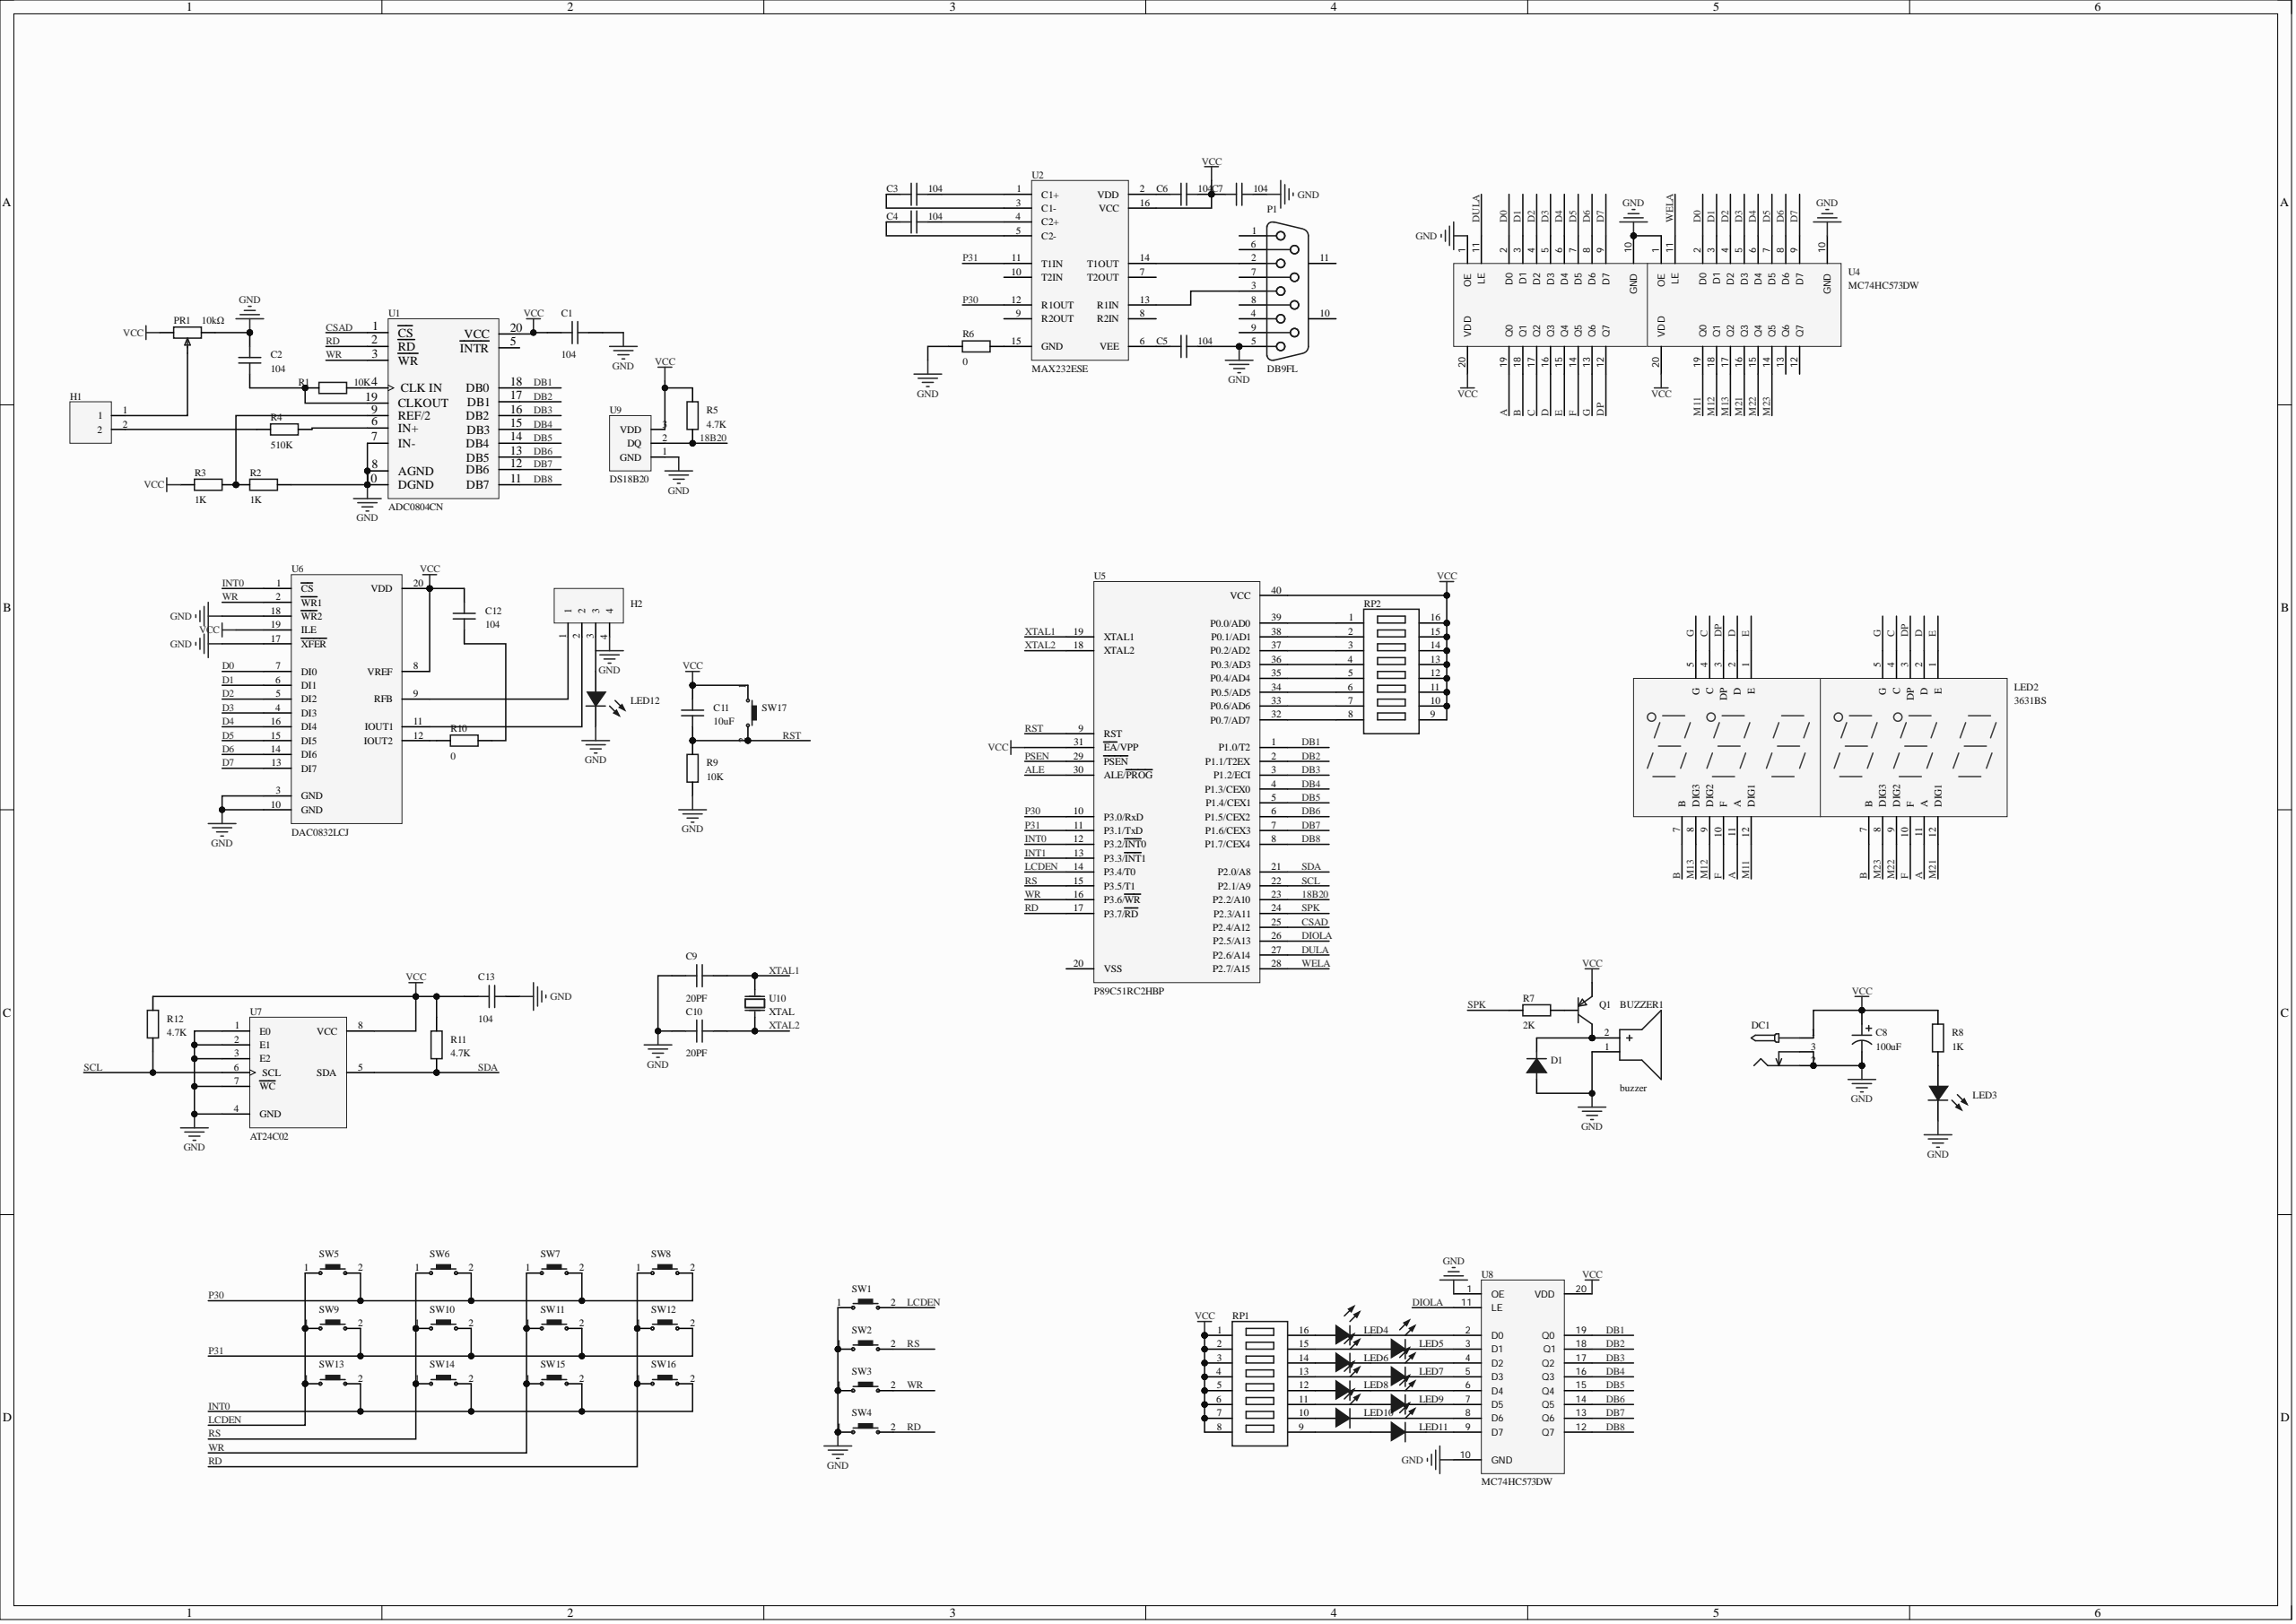Circuit board | Altium Designer | 74 parts | 97 nets
Bill of materials:
Comment,Description,Designator,Footprint,LibRef,Quantity
"buzzer","","BUZZER1","BUZ-TH_BD12.0-P6.00-D0.9-RD","buzzer","1"
"104","","C1, C2, C3, C4, C5, C6, C7, C12, C13","C0603","CAP_0603","9"
"100uF","Capacitance: 10uF; tolerance: ±20%; rated voltage: 50V; ripple current: 120mA@100KHz; equivalent series resistance (ESR): 1.6Ω;","C8","CAP-TH_BD5.0-P2.00-D0.8-FD-10UF50VC110GL","10UF50VC110GL","1"
"20PF","","C9, C10","C0603","CAP_0603","2"
"10uF","","C11","C0603","CAP_0603","1"
"","","D1","DO_1N4007","D_1N4007A","1"
"","","DC1","DC-005_2.5","DC-005_2.5","1"
"","","H1","HDR-TH_2P-P2.54-V-M-1","HDR-M_2.54_1x2P","1"
"","","H2","HDR-TH_4P-P2.54-V-M","HDR-M_2.54_1x4P","1"
"3631BS","Digit count: 3; luminous colour: blue; LED polarity: common anode; digit/letter size (inch): 0.56;","LED1, LED2","LED-SEG-TH_11P-L37.5-W19.0-P2.54-LS15.2-BL_1","3631BS","2"
"","","LED3, LED4, LED5, LED6, LED7, LED8, LED9, LED10, LED11, LED12","LED_0603","LED_0603-B","10"
"DB9FL","","P1","DB9-TH_DB9F","DB9FL","1"
"10kΩ","","PR1","R_3296","R_3296","1"
"","","Q1","S8550P_TO-92","S8550_TO_PNP","1"
"10K","","R1, R9","R0603","Res_0603","2"
"1K","","R2, R3, R8","R0603","Res_0603","3"
"510K","","R4","R0603","Res_0603","1"
"4.7K","","R5, R11, R12","R0603","Res_0603","3"
"0","","R6, R10","R0603","Res_0603","2"
"2K","","R7","R0603","Res_0603","1"
"","","RP1, RP2","DIP-16_L20.3-W10.2-P2.54-LS7.6-BL","paizu","2"
"","","SW1, SW2, SW3, SW4, SW5, SW6, SW7, SW8, SW9, SW10, SW11, SW12, SW13, SW14, SW15, SW16, SW17","Key_SMD_3x4x2","Key_SMD_3x4x2","17"
"ADC0804CN","","U1","ADC0804CN","ADC0804CN","1"
"MAX232ESE","RS232","U2","","MAX232ESE","1"
"MC74HC573DW","","U3, U4, U8","","MC74HC573DW","3"
"P89C51RC2HBP","","U5","","P89C51RC2HBP","1"
"DAC0832LCJ","","U6","J20A","DAC0832LCJ","1"
"AT24C02","","U7","","M24C02BN6","1"
"DS18B20","","U9","TO-92-3_L4.9-W3.7-P1.27-L","DS18B20","1"
"32768/10ppm/12.5pF","","U10","osc-smd_l3.2-w1.5","32768/10ppm/12.5pF","1"
Netlist (Protel format):
[
BUZZER1
BUZ-TH_BD12.0-P6.00-D0.9-RD
buzzer



]
[
C1
C0603
104



]
[
C2
C0603
104



]
[
C3
C0603
104



]
[
C4
C0603
104



]
[
C5
C0603
104



]
[
C6
C0603
104



]
[
C7
C0603
104



]
[
C8
CAP-TH_BD5.0-P2.00-D0.8-FD-10UF50VC110GL
100uF



]
[
C9
C0603
20PF



]
[
C10
C0603
20PF



]
[
C11
C0603
10uF



]
[
C12
C0603
104



]
[
C13
C0603
104



]
[
D1
DO_1N4007




]
[
DC1
DC-005_2.5




]
[
H1
HDR-TH_2P-P2.54-V-M-1




]
[
H2
HDR-TH_4P-P2.54-V-M




]
[
LED1
LED-SEG-TH_11P-L37.5-W19.0-P2.54-LS15.2-BL_1
3631BS



]
[
LED2
LED-SEG-TH_11P-L37.5-W19.0-P2.54-LS15.2-BL_1
3631BS



]
[
LED3
LED_0603




]
[
LED4
LED_0603




]
[
LED5
LED_0603




]
[
LED6
LED_0603




]
[
LED7
LED_0603




]
[
LED8
LED_0603




]
[
LED9
LED_0603




]
[
LED10
LED_0603




]
[
LED11
LED_0603




]
[
LED12
LED_0603




]
[
P1
DB9-TH_DB9F
DB9FL



]
[
PR1
R_3296
10kΩ



]
[
Q1
S8550P_TO-92




]
[
R1
R0603
10K



]
[
R2
R0603
1K



]
[
R3
R0603
1K



]
[
R4
R0603
510K



]
[
R5
R0603
4.7K



]
[
R6
R0603
0



]
[
R7
R0603
2K



]
[
R8
R0603
1K



]
[
R9
R0603
10K



]
[
R10
R0603
0



]
[
R11
R0603
4.7K



]
[
R12
R0603
4.7K



]
[
RP1
DIP-16_L20.3-W10.2-P2.54-LS7.6-BL




]
[
RP2
DIP-16_L20.3-W10.2-P2.54-LS7.6-BL




]
[
SW1
Key_SMD_3x4x2




]
[
SW2
Key_SMD_3x4x2




]
[
SW3
Key_SMD_3x4x2




]
[
SW4
Key_SMD_3x4x2




]
[
SW5
Key_SMD_3x4x2




]
[
SW6
Key_SMD_3x4x2




]
[
SW7
Key_SMD_3x4x2




]
[
SW8
Key_SMD_3x4x2




]
[
SW9
Key_SMD_3x4x2




]
[
SW10
Key_SMD_3x4x2




]
[
SW11
Key_SMD_3x4x2




]
[
SW12
Key_SMD_3x4x2




]
[
SW13
Key_SMD_3x4x2




]
[
SW14
Key_SMD_3x4x2




]
[
SW15
Key_SMD_3x4x2




]
[
SW16
Key_SMD_3x4x2




]
[
SW17
Key_SMD_3x4x2




]
[
U1
ADC0804CN
ADC0804CN



]
[
U2

MAX232ESE



]
[
U3

MC74HC573DW



]
[
U4

MC74HC573DW



]
[
U5

P89C51RC2HBP



]
[
U6
J20A
DAC0832LCJ



]
[
U7

AT24C02



]
[
U8

MC74HC573DW



]
[
U9
TO-92-3_L4.9-W3.7-P1.27-L
DS18B20



]
[
U10
osc-smd_l3.2-w1.5
32768/10ppm/12.5pF



]
(
XTAL2
C10-2
U5-18
U10-1
)
(
XTAL1
C9-2
U5-19
U10-2
)
(
WR
SW3-2
SW7-1
SW11-1
SW15-1
U1-3
U5-16
U6-2
)
(
WELA
U4-11
U5-28
)
(
VCC
C1-1
C6-1
C7-2
C8-1
C11-2
C12-2
C13-1
DC1-1
PR1-1
Q1-1
R3-1
R5-2
R8-2
R11-2
R12-2
RP1-1
RP1-2
RP1-3
RP1-4
RP1-5
RP1-6
RP1-7
RP1-8
RP2-9
RP2-10
RP2-11
RP2-12
RP2-13
RP2-14
RP2-15
RP2-16
SW17-1
U1-20
U2-16
U3-20
U4-20
U5-31
U5-40
U6-8
U6-19
U6-20
U7-8
U8-20
U9-3
)
(
SPK
R7-1
U5-24
)
(
SDA
R11-1
U5-21
U7-5
)
(
SCL
R12-1
U5-22
U7-6
)
(
RST
C11-1
R9-2
SW17-2
U5-9
)
(
RS
SW2-2
SW6-1
SW10-1
SW14-1
U5-15
)
(
RD
SW4-2
SW8-1
SW12-1
SW16-1
U1-2
U5-17
)
(
P31
SW9-2
SW10-2
SW11-2
SW12-2
U2-11
U5-11
)
(
P30
SW5-2
SW6-2
SW7-2
SW8-2
U2-12
U5-10
)
(
NetRP2_8
RP2-8
U5-32
)
(
NetRP2_7
RP2-7
U5-33
)
(
NetRP2_6
RP2-6
U5-34
)
(
NetRP2_5
RP2-5
U5-35
)
(
NetRP2_4
RP2-4
U5-36
)
(
NetRP2_3
RP2-3
U5-37
)
(
NetRP2_2
RP2-2
U5-38
)
(
NetRP2_1
RP2-1
U5-39
)
(
NetR10_1
R10-1
U6-12
)
(
NetR6_2
R6-2
U2-15
)
(
NetR4_2
R4-2
U1-6
)
(
NetR2_1
R2-1
R3-2
U1-9
)
(
NetR1_2
R1-2
U1-4
)
(
NetQ1_2
Q1-2
R7-2
)
(
NetP1_3
P1-3
U2-13
)
(
NetP1_2
P1-2
U2-14
)
(
NetLED11_2
LED11-2
RP1-9
)
(
NetLED11_1
LED11-1
U8-9
)
(
NetLED10_2
LED10-2
RP1-10
)
(
NetLED10_1
LED10-1
U8-8
)
(
NetLED9_2
LED9-2
RP1-11
)
(
NetLED9_1
LED9-1
U8-7
)
(
NetLED8_2
LED8-2
RP1-12
)
(
NetLED8_1
LED8-1
U8-6
)
(
NetLED7_2
LED7-2
RP1-13
)
(
NetLED7_1
LED7-1
U8-5
)
(
NetLED6_2
LED6-2
RP1-14
)
(
NetLED6_1
LED6-1
U8-4
)
(
NetLED5_2
LED5-2
RP1-15
)
(
NetLED5_1
LED5-1
U8-3
)
(
NetLED4_2
LED4-2
RP1-16
)
(
NetLED4_1
LED4-1
U8-2
)
(
NetLED3_2
LED3-2
R8-1
)
(
NetH2_3
H2-3
LED12-2
)
(
NetH2_2
H2-2
U6-11
)
(
NetH2_1
H2-1
U6-9
)
(
NetH1_2
H1-2
R4-1
)
(
NetH1_1
H1-1
PR1-2
)
(
NetC12_1
C12-1
R10-2
)
(
NetC6_2
C6-2
U2-2
)
(
NetC5_2
C5-2
U2-6
)
(
NetC4_2
C4-2
U2-5
)
(
NetC4_1
C4-1
U2-4
)
(
NetC3_2
C3-2
U2-3
)
(
NetC3_1
C3-1
U2-1
)
(
NetC2_1
C2-1
R1-1
U1-19
)
(
NetBUZZER1_2
BUZZER1-2
D1-1
Q1-3
)
(
M23
LED2-8
U4-14
)
(
M22
LED2-9
U4-15
)
(
M21
LED2-12
U4-16
)
(
M13
LED1-8
U4-17
)
(
M12
LED1-9
U4-18
)
(
M11
LED1-12
U4-19
)
(
LCDEN
SW1-2
SW5-1
SW9-1
SW13-1
U5-14
)
(
INT0
SW13-2
SW14-2
SW15-2
SW16-2
U5-12
U6-1
)
(
GND
BUZZER1-1
C1-2
C2-2
C5-1
C7-1
C8-2
C9-1
C10-1
C13-2
D1-2
DC1-2
DC1-3
H2-4
LED3-1
LED12-1
P1-5
PR1-3
R2-2
R6-1
R9-1
SW1-1
SW2-1
SW3-1
SW4-1
U1-7
U1-8
U1-10
U3-1
U3-10
U4-1
U4-10
U6-3
U6-10
U6-17
U6-18
U7-1
U7-2
U7-3
U7-4
U7-7
U8-1
U8-10
U9-1
)
(
G
LED1-5
LED2-5
U3-13
)
(
F
LED1-10
LED2-10
U3-14
)
(
E
LED1-1
LED2-1
U3-15
)
(
DULA
U3-11
U5-27
)
(
DP
LED1-3
LED2-3
U3-12
)
(
DIOLA
U5-26
U8-11
)
(
DB8
U1-11
U5-8
U8-12
)
(
DB7
U1-12
U5-7
U8-13
)
(
DB6
U1-13
U5-6
U8-14
)
(
DB5
U1-14
U5-5
U8-15
)
(
DB4
U1-15
U5-4
U8-16
)
(
DB3
U1-16
U5-3
U8-17
)
(
DB2
U1-17
U5-2
U8-18
)
(
DB1
U1-18
U5-1
U8-19
)
(
D7
U3-9
U4-9
U6-13
)
(
D6
U3-8
U4-8
U6-14
)
(
D5
U3-7
U4-7
U6-15
)
(
D4
U3-6
U4-6
U6-16
)
(
D3
U3-5
U4-5
U6-4
)
(
D2
U3-4
U4-4
U6-5
)
(
D1
U3-3
U4-3
U6-6
)
(
D0
U3-2
U4-2
U6-7
)
(
D
LED1-2
LED2-2
U3-16
)
(
CSAD
U1-1
U5-25
)
(
C
LED1-4
LED2-4
U3-17
)
(
B
LED1-7
LED2-7
U3-18
)
(
A
LED1-11
LED2-11
U3-19
)
(
18B20
R5-1
U5-23
U9-2
)